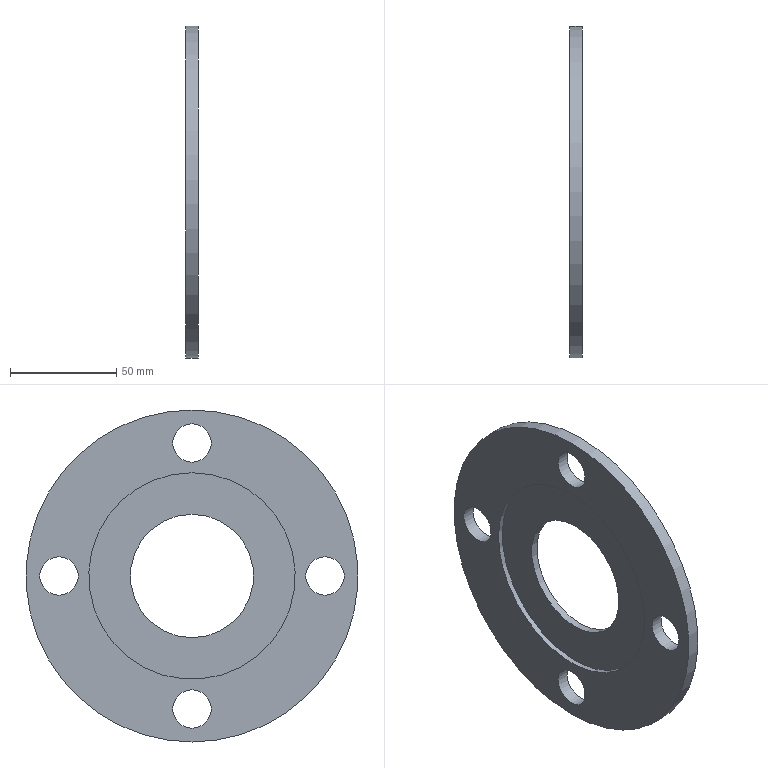Part | STEP file | JBJ-P-1008-01 | 1 solid | 10 faces | box 6 x 156 x 156 mm | volume 80852 mm3 | cylinder 7 | plane 3 | commonest cylinder face diameters 18 x4 58 x1 97 x1 156 x1
STEP:
#1=CARTESIAN_POINT('',(6.,0.,-29.));
#2=VERTEX_POINT('',#1);
#3=CARTESIAN_POINT('',(6.,0.,0.));
#4=DIRECTION('',(1.,0.,0.));
#5=DIRECTION('',(0.,0.,-1.));
#6=AXIS2_PLACEMENT_3D('',#3,#4,#5);
#7=CIRCLE('',#6,29.);
#8=EDGE_CURVE('',#2,#2,#7,.T.);
#9=ORIENTED_EDGE('',*,*,#8,.T.);
#10=EDGE_LOOP('',(#9));
#11=FACE_OUTER_BOUND('',#10,.T.);
#12=CARTESIAN_POINT('',(2.5,0.,29.));
#13=VERTEX_POINT('',#12);
#14=CARTESIAN_POINT('',(2.5,0.,0.));
#15=DIRECTION('',(-1.,0.,0.));
#16=DIRECTION('',(0.,0.,1.));
#17=AXIS2_PLACEMENT_3D('',#14,#15,#16);
#18=CIRCLE('',#17,29.);
#19=EDGE_CURVE('',#13,#13,#18,.T.);
#20=ORIENTED_EDGE('',*,*,#19,.T.);
#21=EDGE_LOOP('',(#20));
#22=FACE_OUTER_BOUND('',#21,.T.);
#23=CARTESIAN_POINT('',(6.,0.,0.));
#24=DIRECTION('',(-1.,0.,0.));
#25=DIRECTION('',(0.,0.,1.));
#26=AXIS2_PLACEMENT_3D('',#23,#24,#25);
#27=CYLINDRICAL_SURFACE('',#26,29.);
#28=ADVANCED_FACE('',(#11,#22),#27,.F.);
#29=CARTESIAN_POINT('',(6.,0.,-71.5));
#30=VERTEX_POINT('',#29);
#31=CARTESIAN_POINT('',(6.,0.,-62.5));
#32=DIRECTION('',(1.,0.,0.));
#33=DIRECTION('',(0.,0.,-1.));
#34=AXIS2_PLACEMENT_3D('',#31,#32,#33);
#35=CIRCLE('',#34,9.);
#36=EDGE_CURVE('',#30,#30,#35,.T.);
#37=ORIENTED_EDGE('',*,*,#36,.F.);
#38=EDGE_LOOP('',(#37));
#39=FACE_BOUND('',#38,.T.);
#40=CARTESIAN_POINT('',(6.,62.5,-9.));
#41=VERTEX_POINT('',#40);
#42=CARTESIAN_POINT('',(6.,62.5,0.));
#43=DIRECTION('',(1.,0.,0.));
#44=DIRECTION('',(0.,0.,-1.));
#45=AXIS2_PLACEMENT_3D('',#42,#43,#44);
#46=CIRCLE('',#45,9.);
#47=EDGE_CURVE('',#41,#41,#46,.T.);
#48=ORIENTED_EDGE('',*,*,#47,.F.);
#49=EDGE_LOOP('',(#48));
#50=FACE_BOUND('',#49,.T.);
#51=CARTESIAN_POINT('',(6.,0.,-78.));
#52=VERTEX_POINT('',#51);
#53=CARTESIAN_POINT('',(6.,0.,0.));
#54=DIRECTION('',(1.,0.,0.));
#55=DIRECTION('',(0.,0.,-1.));
#56=AXIS2_PLACEMENT_3D('',#53,#54,#55);
#57=CIRCLE('',#56,78.);
#58=EDGE_CURVE('',#52,#52,#57,.T.);
#59=ORIENTED_EDGE('',*,*,#58,.T.);
#60=EDGE_LOOP('',(#59));
#61=FACE_OUTER_BOUND('',#60,.T.);
#62=ORIENTED_EDGE('',*,*,#8,.F.);
#63=EDGE_LOOP('',(#62));
#64=FACE_BOUND('',#63,.T.);
#65=CARTESIAN_POINT('',(6.,0.,53.5));
#66=VERTEX_POINT('',#65);
#67=CARTESIAN_POINT('',(6.,0.,62.5));
#68=DIRECTION('',(1.,0.,0.));
#69=DIRECTION('',(0.,0.,-1.));
#70=AXIS2_PLACEMENT_3D('',#67,#68,#69);
#71=CIRCLE('',#70,9.);
#72=EDGE_CURVE('',#66,#66,#71,.T.);
#73=ORIENTED_EDGE('',*,*,#72,.F.);
#74=EDGE_LOOP('',(#73));
#75=FACE_BOUND('',#74,.T.);
#76=CARTESIAN_POINT('',(6.,-62.5,-9.));
#77=VERTEX_POINT('',#76);
#78=CARTESIAN_POINT('',(6.,-62.5,0.));
#79=DIRECTION('',(1.,0.,0.));
#80=DIRECTION('',(0.,0.,-1.));
#81=AXIS2_PLACEMENT_3D('',#78,#79,#80);
#82=CIRCLE('',#81,9.);
#83=EDGE_CURVE('',#77,#77,#82,.T.);
#84=ORIENTED_EDGE('',*,*,#83,.F.);
#85=EDGE_LOOP('',(#84));
#86=FACE_BOUND('',#85,.T.);
#87=CARTESIAN_POINT('',(6.,0.,0.));
#88=DIRECTION('',(1.,0.,0.));
#89=DIRECTION('',(0.,0.,-1.));
#90=AXIS2_PLACEMENT_3D('',#87,#88,#89);
#91=PLANE('',#90);
#92=ADVANCED_FACE('',(#39,#50,#61,#64,#75,#86),#91,.T.);
#93=CARTESIAN_POINT('',(0.,0.,48.5));
#94=VERTEX_POINT('',#93);
#95=CARTESIAN_POINT('',(0.,0.,0.));
#96=DIRECTION('',(-1.,0.,0.));
#97=DIRECTION('',(0.,0.,1.));
#98=AXIS2_PLACEMENT_3D('',#95,#96,#97);
#99=CIRCLE('',#98,48.5);
#100=EDGE_CURVE('',#94,#94,#99,.T.);
#101=ORIENTED_EDGE('',*,*,#100,.F.);
#102=EDGE_LOOP('',(#101));
#103=FACE_BOUND('',#102,.T.);
#104=CARTESIAN_POINT('',(0.,0.,-78.));
#105=VERTEX_POINT('',#104);
#106=CARTESIAN_POINT('',(0.,0.,0.));
#107=DIRECTION('',(1.,0.,0.));
#108=DIRECTION('',(0.,0.,-1.));
#109=AXIS2_PLACEMENT_3D('',#106,#107,#108);
#110=CIRCLE('',#109,78.);
#111=EDGE_CURVE('',#105,#105,#110,.T.);
#112=ORIENTED_EDGE('',*,*,#111,.F.);
#113=EDGE_LOOP('',(#112));
#114=FACE_OUTER_BOUND('',#113,.T.);
#115=CARTESIAN_POINT('',(0.,62.5,-9.));
#116=VERTEX_POINT('',#115);
#117=CARTESIAN_POINT('',(0.,62.5,0.));
#118=DIRECTION('',(1.,0.,0.));
#119=DIRECTION('',(0.,0.,-1.));
#120=AXIS2_PLACEMENT_3D('',#117,#118,#119);
#121=CIRCLE('',#120,9.);
#122=EDGE_CURVE('',#116,#116,#121,.T.);
#123=ORIENTED_EDGE('',*,*,#122,.T.);
#124=EDGE_LOOP('',(#123));
#125=FACE_BOUND('',#124,.T.);
#126=CARTESIAN_POINT('',(0.,0.,53.5));
#127=VERTEX_POINT('',#126);
#128=CARTESIAN_POINT('',(0.,0.,62.5));
#129=DIRECTION('',(1.,0.,0.));
#130=DIRECTION('',(0.,0.,-1.));
#131=AXIS2_PLACEMENT_3D('',#128,#129,#130);
#132=CIRCLE('',#131,9.);
#133=EDGE_CURVE('',#127,#127,#132,.T.);
#134=ORIENTED_EDGE('',*,*,#133,.T.);
#135=EDGE_LOOP('',(#134));
#136=FACE_BOUND('',#135,.T.);
#137=CARTESIAN_POINT('',(0.,0.,-71.5));
#138=VERTEX_POINT('',#137);
#139=CARTESIAN_POINT('',(0.,0.,-62.5));
#140=DIRECTION('',(1.,0.,0.));
#141=DIRECTION('',(0.,0.,-1.));
#142=AXIS2_PLACEMENT_3D('',#139,#140,#141);
#143=CIRCLE('',#142,9.);
#144=EDGE_CURVE('',#138,#138,#143,.T.);
#145=ORIENTED_EDGE('',*,*,#144,.T.);
#146=EDGE_LOOP('',(#145));
#147=FACE_BOUND('',#146,.T.);
#148=CARTESIAN_POINT('',(0.,-62.5,-9.));
#149=VERTEX_POINT('',#148);
#150=CARTESIAN_POINT('',(0.,-62.5,0.));
#151=DIRECTION('',(1.,0.,0.));
#152=DIRECTION('',(0.,0.,-1.));
#153=AXIS2_PLACEMENT_3D('',#150,#151,#152);
#154=CIRCLE('',#153,9.);
#155=EDGE_CURVE('',#149,#149,#154,.T.);
#156=ORIENTED_EDGE('',*,*,#155,.T.);
#157=EDGE_LOOP('',(#156));
#158=FACE_BOUND('',#157,.T.);
#159=CARTESIAN_POINT('',(0.,0.,0.));
#160=DIRECTION('',(1.,0.,0.));
#161=DIRECTION('',(0.,0.,-1.));
#162=AXIS2_PLACEMENT_3D('',#159,#160,#161);
#163=PLANE('',#162);
#164=ADVANCED_FACE('',(#103,#114,#125,#136,#147,#158),#163,.F.);
#165=ORIENTED_EDGE('',*,*,#58,.F.);
#166=EDGE_LOOP('',(#165));
#167=FACE_OUTER_BOUND('',#166,.T.);
#168=ORIENTED_EDGE('',*,*,#111,.T.);
#169=EDGE_LOOP('',(#168));
#170=FACE_OUTER_BOUND('',#169,.T.);
#171=CARTESIAN_POINT('',(6.,0.,0.));
#172=DIRECTION('',(-1.,0.,0.));
#173=DIRECTION('',(0.,0.,1.));
#174=AXIS2_PLACEMENT_3D('',#171,#172,#173);
#175=CYLINDRICAL_SURFACE('',#174,78.);
#176=ADVANCED_FACE('',(#167,#170),#175,.T.);
#177=ORIENTED_EDGE('',*,*,#47,.T.);
#178=EDGE_LOOP('',(#177));
#179=FACE_OUTER_BOUND('',#178,.T.);
#180=ORIENTED_EDGE('',*,*,#122,.F.);
#181=EDGE_LOOP('',(#180));
#182=FACE_OUTER_BOUND('',#181,.T.);
#183=CARTESIAN_POINT('',(6.,62.5,0.));
#184=DIRECTION('',(-1.,0.,0.));
#185=DIRECTION('',(0.,0.,1.));
#186=AXIS2_PLACEMENT_3D('',#183,#184,#185);
#187=CYLINDRICAL_SURFACE('',#186,9.);
#188=ADVANCED_FACE('',(#179,#182),#187,.F.);
#189=ORIENTED_EDGE('',*,*,#72,.T.);
#190=EDGE_LOOP('',(#189));
#191=FACE_OUTER_BOUND('',#190,.T.);
#192=ORIENTED_EDGE('',*,*,#133,.F.);
#193=EDGE_LOOP('',(#192));
#194=FACE_OUTER_BOUND('',#193,.T.);
#195=CARTESIAN_POINT('',(6.,0.,62.5));
#196=DIRECTION('',(-1.,0.,0.));
#197=DIRECTION('',(0.,0.,1.));
#198=AXIS2_PLACEMENT_3D('',#195,#196,#197);
#199=CYLINDRICAL_SURFACE('',#198,9.);
#200=ADVANCED_FACE('',(#191,#194),#199,.F.);
#201=ORIENTED_EDGE('',*,*,#36,.T.);
#202=EDGE_LOOP('',(#201));
#203=FACE_OUTER_BOUND('',#202,.T.);
#204=ORIENTED_EDGE('',*,*,#144,.F.);
#205=EDGE_LOOP('',(#204));
#206=FACE_OUTER_BOUND('',#205,.T.);
#207=CARTESIAN_POINT('',(6.,0.,-62.5));
#208=DIRECTION('',(-1.,0.,0.));
#209=DIRECTION('',(0.,0.,1.));
#210=AXIS2_PLACEMENT_3D('',#207,#208,#209);
#211=CYLINDRICAL_SURFACE('',#210,9.);
#212=ADVANCED_FACE('',(#203,#206),#211,.F.);
#213=ORIENTED_EDGE('',*,*,#83,.T.);
#214=EDGE_LOOP('',(#213));
#215=FACE_OUTER_BOUND('',#214,.T.);
#216=ORIENTED_EDGE('',*,*,#155,.F.);
#217=EDGE_LOOP('',(#216));
#218=FACE_OUTER_BOUND('',#217,.T.);
#219=CARTESIAN_POINT('',(6.,-62.5,0.));
#220=DIRECTION('',(-1.,0.,0.));
#221=DIRECTION('',(0.,0.,1.));
#222=AXIS2_PLACEMENT_3D('',#219,#220,#221);
#223=CYLINDRICAL_SURFACE('',#222,9.);
#224=ADVANCED_FACE('',(#215,#218),#223,.F.);
#225=CARTESIAN_POINT('',(2.5,0.,48.5));
#226=VERTEX_POINT('',#225);
#227=CARTESIAN_POINT('',(2.5,0.,0.));
#228=DIRECTION('',(-1.,0.,0.));
#229=DIRECTION('',(0.,0.,1.));
#230=AXIS2_PLACEMENT_3D('',#227,#228,#229);
#231=CIRCLE('',#230,48.5);
#232=EDGE_CURVE('',#226,#226,#231,.T.);
#233=ORIENTED_EDGE('',*,*,#232,.F.);
#234=EDGE_LOOP('',(#233));
#235=FACE_OUTER_BOUND('',#234,.T.);
#236=ORIENTED_EDGE('',*,*,#100,.T.);
#237=EDGE_LOOP('',(#236));
#238=FACE_OUTER_BOUND('',#237,.T.);
#239=CARTESIAN_POINT('',(2.5,0.,0.));
#240=DIRECTION('',(-1.,0.,0.));
#241=DIRECTION('',(0.,0.,1.));
#242=AXIS2_PLACEMENT_3D('',#239,#240,#241);
#243=CYLINDRICAL_SURFACE('',#242,48.5);
#244=ADVANCED_FACE('',(#235,#238),#243,.F.);
#245=ORIENTED_EDGE('',*,*,#19,.F.);
#246=EDGE_LOOP('',(#245));
#247=FACE_BOUND('',#246,.T.);
#248=ORIENTED_EDGE('',*,*,#232,.T.);
#249=EDGE_LOOP('',(#248));
#250=FACE_OUTER_BOUND('',#249,.T.);
#251=CARTESIAN_POINT('',(2.5,0.,0.));
#252=DIRECTION('',(-1.,0.,0.));
#253=DIRECTION('',(0.,0.,1.));
#254=AXIS2_PLACEMENT_3D('',#251,#252,#253);
#255=PLANE('',#254);
#256=ADVANCED_FACE('',(#247,#250),#255,.T.);
#257=CLOSED_SHELL('',(#28,#92,#164,#176,#188,#200,#212,#224,#244,#256));
#258=MANIFOLD_SOLID_BREP('',#257);
#259=CARTESIAN_POINT('',(0.,0.,0.));
#260=DIRECTION('',(0.,0.,1.));
#261=DIRECTION('',(1.,0.,0.));
#262=AXIS2_PLACEMENT_3D('',#259,#260,#261);
#263=(LENGTH_UNIT()NAMED_UNIT(*)SI_UNIT(.MILLI.,.METRE.));
#264=UNCERTAINTY_MEASURE_WITH_UNIT(LENGTH_MEASURE(0.00001),#263,'','');
#265=(NAMED_UNIT(*)PLANE_ANGLE_UNIT()SI_UNIT($,.RADIAN.));
#266=(NAMED_UNIT(*)SI_UNIT($,.STERADIAN.)SOLID_ANGLE_UNIT());
#267=(GEOMETRIC_REPRESENTATION_CONTEXT(3)GLOBAL_UNCERTAINTY_ASSIGNED_CONTEXT((#264))GLOBAL_UNIT_ASSIGNED_CONTEXT((#263,#265,#266))REPRESENTATION_CONTEXT('',''));
#268=ADVANCED_BREP_SHAPE_REPRESENTATION('',(#258,#262),#267);